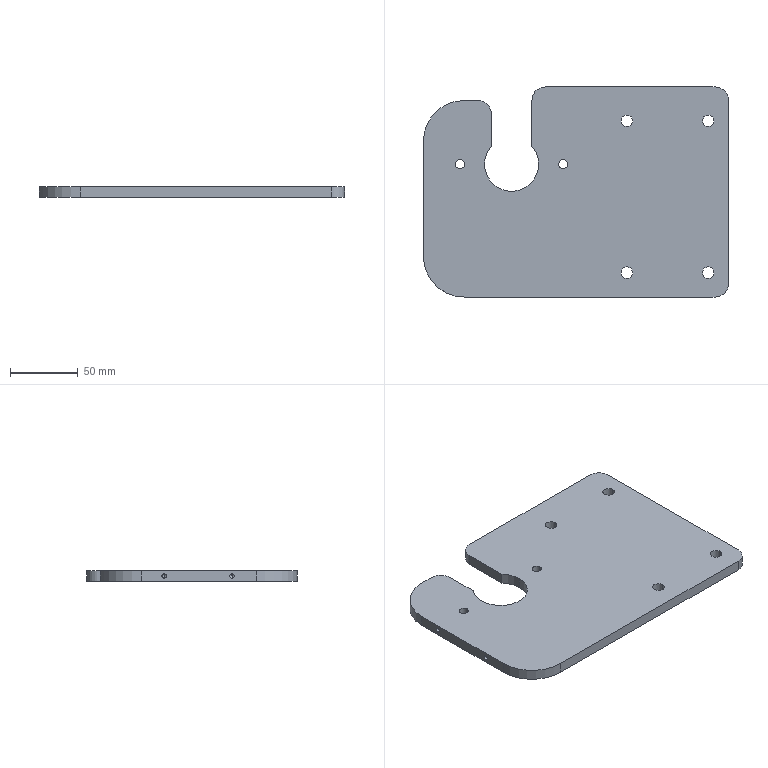Part | SolidWorks | features BaseBody 1 | 1 solid | 38 faces | box 225 x 155 x 8 mm | volume 249192 mm3 | cylinder 25 | plane 9 | cone 4 | commonest cylinder face diameters 8.5 x8 3.3 x4 6.8 x4 20 x4 40 x3 60 x2
STEP:
#1=CARTESIAN_POINT('',(-67.5,20.5,0.));
#2=VERTEX_POINT('',#1);
#3=CARTESIAN_POINT('',(-27.5,20.5,0.));
#4=VERTEX_POINT('',#3);
#5=CARTESIAN_POINT('',(-47.5,20.5,0.));
#6=DIRECTION('',(0.,0.,1.));
#7=DIRECTION('',(1.,0.,0.));
#8=AXIS2_PLACEMENT_3D('',#5,#6,#7);
#9=CIRCLE('',#8,20.);
#10=EDGE_CURVE('',#2,#4,#9,.T.);
#11=ORIENTED_EDGE('',*,*,#10,.F.);
#12=CARTESIAN_POINT('',(-67.5,20.5,8.));
#13=VERTEX_POINT('',#12);
#14=CARTESIAN_POINT('',(-67.5,20.5,0.));
#15=DIRECTION('',(0.,0.,1.));
#16=VECTOR('',#15,1000.);
#17=LINE('',#14,#16);
#18=EDGE_CURVE('',#2,#13,#17,.T.);
#19=ORIENTED_EDGE('',*,*,#18,.T.);
#20=CARTESIAN_POINT('',(-27.5,20.5,8.));
#21=VERTEX_POINT('',#20);
#22=CARTESIAN_POINT('',(-47.5,20.5,8.));
#23=DIRECTION('',(0.,0.,1.));
#24=DIRECTION('',(1.,0.,0.));
#25=AXIS2_PLACEMENT_3D('',#22,#23,#24);
#26=CIRCLE('',#25,20.);
#27=EDGE_CURVE('',#13,#21,#26,.T.);
#28=ORIENTED_EDGE('',*,*,#27,.T.);
#29=CARTESIAN_POINT('',(-27.5,20.5,0.));
#30=DIRECTION('',(0.,0.,1.));
#31=VECTOR('',#30,1000.);
#32=LINE('',#29,#31);
#33=EDGE_CURVE('',#4,#21,#32,.T.);
#34=ORIENTED_EDGE('',*,*,#33,.F.);
#35=EDGE_LOOP('',(#11,#19,#28,#34));
#36=FACE_OUTER_BOUND('',#35,.T.);
#37=CARTESIAN_POINT('',(-47.5,20.5,0.));
#38=DIRECTION('',(0.,0.,1.));
#39=DIRECTION('',(1.,0.,0.));
#40=AXIS2_PLACEMENT_3D('',#37,#38,#39);
#41=CYLINDRICAL_SURFACE('',#40,20.);
#42=ADVANCED_FACE('',(#36),#41,.F.);
#43=CARTESIAN_POINT('',(-32.5,33.729,0.));
#44=VERTEX_POINT('',#43);
#45=CARTESIAN_POINT('',(-47.5,20.5,0.));
#46=DIRECTION('',(0.,0.,1.));
#47=DIRECTION('',(1.,0.,0.));
#48=AXIS2_PLACEMENT_3D('',#45,#46,#47);
#49=CIRCLE('',#48,20.);
#50=EDGE_CURVE('',#4,#44,#49,.T.);
#51=ORIENTED_EDGE('',*,*,#50,.F.);
#52=ORIENTED_EDGE('',*,*,#33,.T.);
#53=CARTESIAN_POINT('',(-32.5,33.729,8.));
#54=VERTEX_POINT('',#53);
#55=CARTESIAN_POINT('',(-47.5,20.5,8.));
#56=DIRECTION('',(0.,0.,1.));
#57=DIRECTION('',(1.,0.,0.));
#58=AXIS2_PLACEMENT_3D('',#55,#56,#57);
#59=CIRCLE('',#58,20.);
#60=EDGE_CURVE('',#21,#54,#59,.T.);
#61=ORIENTED_EDGE('',*,*,#60,.T.);
#62=CARTESIAN_POINT('',(-32.5,33.729,8.));
#63=DIRECTION('',(0.,0.,-1.));
#64=VECTOR('',#63,1000.);
#65=LINE('',#62,#64);
#66=EDGE_CURVE('',#54,#44,#65,.T.);
#67=ORIENTED_EDGE('',*,*,#66,.T.);
#68=EDGE_LOOP('',(#51,#52,#61,#67));
#69=FACE_OUTER_BOUND('',#68,.T.);
#70=CARTESIAN_POINT('',(-47.5,20.5,0.));
#71=DIRECTION('',(0.,0.,1.));
#72=DIRECTION('',(1.,0.,0.));
#73=AXIS2_PLACEMENT_3D('',#70,#71,#72);
#74=CYLINDRICAL_SURFACE('',#73,20.);
#75=ADVANCED_FACE('',(#69),#74,.F.);
#76=CARTESIAN_POINT('',(33.25,52.5,8.));
#77=VERTEX_POINT('',#76);
#78=CARTESIAN_POINT('',(41.75,52.5,8.));
#79=VERTEX_POINT('',#78);
#80=CARTESIAN_POINT('',(37.5,52.5,8.));
#81=DIRECTION('',(0.,0.,1.));
#82=DIRECTION('',(-1.,0.,0.));
#83=AXIS2_PLACEMENT_3D('',#80,#81,#82);
#84=CIRCLE('',#83,4.25);
#85=EDGE_CURVE('',#77,#79,#84,.T.);
#86=ORIENTED_EDGE('',*,*,#85,.T.);
#87=CARTESIAN_POINT('',(41.75,52.5,0.));
#88=VERTEX_POINT('',#87);
#89=CARTESIAN_POINT('',(41.75,52.5,0.));
#90=DIRECTION('',(0.,0.,-1.));
#91=VECTOR('',#90,1000.);
#92=LINE('',#89,#91);
#93=EDGE_CURVE('',#79,#88,#92,.T.);
#94=ORIENTED_EDGE('',*,*,#93,.T.);
#95=CARTESIAN_POINT('',(33.25,52.5,0.));
#96=VERTEX_POINT('',#95);
#97=CARTESIAN_POINT('',(37.5,52.5,0.));
#98=DIRECTION('',(0.,0.,1.));
#99=DIRECTION('',(-1.,0.,0.));
#100=AXIS2_PLACEMENT_3D('',#97,#98,#99);
#101=CIRCLE('',#100,4.25);
#102=EDGE_CURVE('',#96,#88,#101,.T.);
#103=ORIENTED_EDGE('',*,*,#102,.F.);
#104=CARTESIAN_POINT('',(33.25,52.5,0.));
#105=DIRECTION('',(0.,0.,-1.));
#106=VECTOR('',#105,1000.);
#107=LINE('',#104,#106);
#108=EDGE_CURVE('',#77,#96,#107,.T.);
#109=ORIENTED_EDGE('',*,*,#108,.F.);
#110=EDGE_LOOP('',(#86,#94,#103,#109));
#111=FACE_OUTER_BOUND('',#110,.T.);
#112=CARTESIAN_POINT('',(37.5,52.5,0.));
#113=DIRECTION('',(0.,0.,-1.));
#114=DIRECTION('',(-1.,0.,0.));
#115=AXIS2_PLACEMENT_3D('',#112,#113,#114);
#116=CYLINDRICAL_SURFACE('',#115,4.25);
#117=ADVANCED_FACE('',(#111),#116,.F.);
#118=CARTESIAN_POINT('',(93.25,-59.5,8.));
#119=VERTEX_POINT('',#118);
#120=CARTESIAN_POINT('',(101.75,-59.5,8.));
#121=VERTEX_POINT('',#120);
#122=CARTESIAN_POINT('',(97.5,-59.5,8.));
#123=DIRECTION('',(0.,0.,1.));
#124=DIRECTION('',(-1.,0.,0.));
#125=AXIS2_PLACEMENT_3D('',#122,#123,#124);
#126=CIRCLE('',#125,4.25);
#127=EDGE_CURVE('',#119,#121,#126,.T.);
#128=ORIENTED_EDGE('',*,*,#127,.T.);
#129=CARTESIAN_POINT('',(101.75,-59.5,0.));
#130=VERTEX_POINT('',#129);
#131=CARTESIAN_POINT('',(101.75,-59.5,0.));
#132=DIRECTION('',(0.,0.,-1.));
#133=VECTOR('',#132,1000.);
#134=LINE('',#131,#133);
#135=EDGE_CURVE('',#121,#130,#134,.T.);
#136=ORIENTED_EDGE('',*,*,#135,.T.);
#137=CARTESIAN_POINT('',(93.25,-59.5,0.));
#138=VERTEX_POINT('',#137);
#139=CARTESIAN_POINT('',(97.5,-59.5,0.));
#140=DIRECTION('',(0.,0.,1.));
#141=DIRECTION('',(-1.,0.,0.));
#142=AXIS2_PLACEMENT_3D('',#139,#140,#141);
#143=CIRCLE('',#142,4.25);
#144=EDGE_CURVE('',#138,#130,#143,.T.);
#145=ORIENTED_EDGE('',*,*,#144,.F.);
#146=CARTESIAN_POINT('',(93.25,-59.5,0.));
#147=DIRECTION('',(0.,0.,-1.));
#148=VECTOR('',#147,1000.);
#149=LINE('',#146,#148);
#150=EDGE_CURVE('',#119,#138,#149,.T.);
#151=ORIENTED_EDGE('',*,*,#150,.F.);
#152=EDGE_LOOP('',(#128,#136,#145,#151));
#153=FACE_OUTER_BOUND('',#152,.T.);
#154=CARTESIAN_POINT('',(97.5,-59.5,0.));
#155=DIRECTION('',(0.,0.,-1.));
#156=DIRECTION('',(-1.,0.,0.));
#157=AXIS2_PLACEMENT_3D('',#154,#155,#156);
#158=CYLINDRICAL_SURFACE('',#157,4.25);
#159=ADVANCED_FACE('',(#153),#158,.F.);
#160=CARTESIAN_POINT('',(33.25,-59.5,8.));
#161=VERTEX_POINT('',#160);
#162=CARTESIAN_POINT('',(41.75,-59.5,8.));
#163=VERTEX_POINT('',#162);
#164=CARTESIAN_POINT('',(37.5,-59.5,8.));
#165=DIRECTION('',(0.,0.,1.));
#166=DIRECTION('',(-1.,0.,0.));
#167=AXIS2_PLACEMENT_3D('',#164,#165,#166);
#168=CIRCLE('',#167,4.25);
#169=EDGE_CURVE('',#161,#163,#168,.T.);
#170=ORIENTED_EDGE('',*,*,#169,.T.);
#171=CARTESIAN_POINT('',(41.75,-59.5,0.));
#172=VERTEX_POINT('',#171);
#173=CARTESIAN_POINT('',(41.75,-59.5,0.));
#174=DIRECTION('',(0.,0.,-1.));
#175=VECTOR('',#174,1000.);
#176=LINE('',#173,#175);
#177=EDGE_CURVE('',#163,#172,#176,.T.);
#178=ORIENTED_EDGE('',*,*,#177,.T.);
#179=CARTESIAN_POINT('',(33.25,-59.5,0.));
#180=VERTEX_POINT('',#179);
#181=CARTESIAN_POINT('',(37.5,-59.5,0.));
#182=DIRECTION('',(0.,0.,1.));
#183=DIRECTION('',(-1.,0.,0.));
#184=AXIS2_PLACEMENT_3D('',#181,#182,#183);
#185=CIRCLE('',#184,4.25);
#186=EDGE_CURVE('',#180,#172,#185,.T.);
#187=ORIENTED_EDGE('',*,*,#186,.F.);
#188=CARTESIAN_POINT('',(33.25,-59.5,0.));
#189=DIRECTION('',(0.,0.,-1.));
#190=VECTOR('',#189,1000.);
#191=LINE('',#188,#190);
#192=EDGE_CURVE('',#161,#180,#191,.T.);
#193=ORIENTED_EDGE('',*,*,#192,.F.);
#194=EDGE_LOOP('',(#170,#178,#187,#193));
#195=FACE_OUTER_BOUND('',#194,.T.);
#196=CARTESIAN_POINT('',(37.5,-59.5,0.));
#197=DIRECTION('',(0.,0.,-1.));
#198=DIRECTION('',(-1.,0.,0.));
#199=AXIS2_PLACEMENT_3D('',#196,#197,#198);
#200=CYLINDRICAL_SURFACE('',#199,4.25);
#201=ADVANCED_FACE('',(#195),#200,.F.);
#202=CARTESIAN_POINT('',(93.25,52.5,8.));
#203=VERTEX_POINT('',#202);
#204=CARTESIAN_POINT('',(101.75,52.5,8.));
#205=VERTEX_POINT('',#204);
#206=CARTESIAN_POINT('',(97.5,52.5,8.));
#207=DIRECTION('',(0.,0.,1.));
#208=DIRECTION('',(-1.,0.,0.));
#209=AXIS2_PLACEMENT_3D('',#206,#207,#208);
#210=CIRCLE('',#209,4.25);
#211=EDGE_CURVE('',#203,#205,#210,.T.);
#212=ORIENTED_EDGE('',*,*,#211,.T.);
#213=CARTESIAN_POINT('',(101.75,52.5,0.));
#214=VERTEX_POINT('',#213);
#215=CARTESIAN_POINT('',(101.75,52.5,0.));
#216=DIRECTION('',(0.,0.,-1.));
#217=VECTOR('',#216,1000.);
#218=LINE('',#215,#217);
#219=EDGE_CURVE('',#205,#214,#218,.T.);
#220=ORIENTED_EDGE('',*,*,#219,.T.);
#221=CARTESIAN_POINT('',(93.25,52.5,0.));
#222=VERTEX_POINT('',#221);
#223=CARTESIAN_POINT('',(97.5,52.5,0.));
#224=DIRECTION('',(0.,0.,1.));
#225=DIRECTION('',(-1.,0.,0.));
#226=AXIS2_PLACEMENT_3D('',#223,#224,#225);
#227=CIRCLE('',#226,4.25);
#228=EDGE_CURVE('',#222,#214,#227,.T.);
#229=ORIENTED_EDGE('',*,*,#228,.F.);
#230=CARTESIAN_POINT('',(93.25,52.5,0.));
#231=DIRECTION('',(0.,0.,-1.));
#232=VECTOR('',#231,1000.);
#233=LINE('',#230,#232);
#234=EDGE_CURVE('',#203,#222,#233,.T.);
#235=ORIENTED_EDGE('',*,*,#234,.F.);
#236=EDGE_LOOP('',(#212,#220,#229,#235));
#237=FACE_OUTER_BOUND('',#236,.T.);
#238=CARTESIAN_POINT('',(97.5,52.5,0.));
#239=DIRECTION('',(0.,0.,-1.));
#240=DIRECTION('',(-1.,0.,0.));
#241=AXIS2_PLACEMENT_3D('',#238,#239,#240);
#242=CYLINDRICAL_SURFACE('',#241,4.25);
#243=ADVANCED_FACE('',(#237),#242,.F.);
#244=CARTESIAN_POINT('',(-88.9,20.5,8.));
#245=VERTEX_POINT('',#244);
#246=CARTESIAN_POINT('',(-82.1,20.5,8.));
#247=VERTEX_POINT('',#246);
#248=CARTESIAN_POINT('',(-85.5,20.5,8.));
#249=DIRECTION('',(0.,0.,1.));
#250=DIRECTION('',(-1.,0.,0.));
#251=AXIS2_PLACEMENT_3D('',#248,#249,#250);
#252=CIRCLE('',#251,3.4);
#253=EDGE_CURVE('',#245,#247,#252,.T.);
#254=ORIENTED_EDGE('',*,*,#253,.T.);
#255=CARTESIAN_POINT('',(-82.1,20.5,0.));
#256=VERTEX_POINT('',#255);
#257=CARTESIAN_POINT('',(-82.1,20.5,0.));
#258=DIRECTION('',(0.,0.,-1.));
#259=VECTOR('',#258,1000.);
#260=LINE('',#257,#259);
#261=EDGE_CURVE('',#247,#256,#260,.T.);
#262=ORIENTED_EDGE('',*,*,#261,.T.);
#263=CARTESIAN_POINT('',(-88.9,20.5,0.));
#264=VERTEX_POINT('',#263);
#265=CARTESIAN_POINT('',(-85.5,20.5,0.));
#266=DIRECTION('',(0.,0.,1.));
#267=DIRECTION('',(-1.,0.,0.));
#268=AXIS2_PLACEMENT_3D('',#265,#266,#267);
#269=CIRCLE('',#268,3.4);
#270=EDGE_CURVE('',#264,#256,#269,.T.);
#271=ORIENTED_EDGE('',*,*,#270,.F.);
#272=CARTESIAN_POINT('',(-88.9,20.5,0.));
#273=DIRECTION('',(0.,0.,-1.));
#274=VECTOR('',#273,1000.);
#275=LINE('',#272,#274);
#276=EDGE_CURVE('',#245,#264,#275,.T.);
#277=ORIENTED_EDGE('',*,*,#276,.F.);
#278=EDGE_LOOP('',(#254,#262,#271,#277));
#279=FACE_OUTER_BOUND('',#278,.T.);
#280=CARTESIAN_POINT('',(-85.5,20.5,0.));
#281=DIRECTION('',(0.,0.,-1.));
#282=DIRECTION('',(-1.,0.,0.));
#283=AXIS2_PLACEMENT_3D('',#280,#281,#282);
#284=CYLINDRICAL_SURFACE('',#283,3.4);
#285=ADVANCED_FACE('',(#279),#284,.F.);
#286=CARTESIAN_POINT('',(-12.9,20.5,8.));
#287=VERTEX_POINT('',#286);
#288=CARTESIAN_POINT('',(-6.1,20.5,8.));
#289=VERTEX_POINT('',#288);
#290=CARTESIAN_POINT('',(-9.5,20.5,8.));
#291=DIRECTION('',(0.,0.,1.));
#292=DIRECTION('',(-1.,0.,0.));
#293=AXIS2_PLACEMENT_3D('',#290,#291,#292);
#294=CIRCLE('',#293,3.4);
#295=EDGE_CURVE('',#287,#289,#294,.T.);
#296=ORIENTED_EDGE('',*,*,#295,.T.);
#297=CARTESIAN_POINT('',(-6.1,20.5,0.));
#298=VERTEX_POINT('',#297);
#299=CARTESIAN_POINT('',(-6.1,20.5,0.));
#300=DIRECTION('',(0.,0.,-1.));
#301=VECTOR('',#300,1000.);
#302=LINE('',#299,#301);
#303=EDGE_CURVE('',#289,#298,#302,.T.);
#304=ORIENTED_EDGE('',*,*,#303,.T.);
#305=CARTESIAN_POINT('',(-12.9,20.5,0.));
#306=VERTEX_POINT('',#305);
#307=CARTESIAN_POINT('',(-9.5,20.5,0.));
#308=DIRECTION('',(0.,0.,1.));
#309=DIRECTION('',(-1.,0.,0.));
#310=AXIS2_PLACEMENT_3D('',#307,#308,#309);
#311=CIRCLE('',#310,3.4);
#312=EDGE_CURVE('',#306,#298,#311,.T.);
#313=ORIENTED_EDGE('',*,*,#312,.F.);
#314=CARTESIAN_POINT('',(-12.9,20.5,0.));
#315=DIRECTION('',(0.,0.,-1.));
#316=VECTOR('',#315,1000.);
#317=LINE('',#314,#316);
#318=EDGE_CURVE('',#287,#306,#317,.T.);
#319=ORIENTED_EDGE('',*,*,#318,.F.);
#320=EDGE_LOOP('',(#296,#304,#313,#319));
#321=FACE_OUTER_BOUND('',#320,.T.);
#322=CARTESIAN_POINT('',(-9.5,20.5,0.));
#323=DIRECTION('',(0.,0.,-1.));
#324=DIRECTION('',(-1.,0.,0.));
#325=AXIS2_PLACEMENT_3D('',#322,#323,#324);
#326=CYLINDRICAL_SURFACE('',#325,3.4);
#327=ADVANCED_FACE('',(#321),#326,.F.);
#328=CARTESIAN_POINT('',(-101.,-29.5,2.35));
#329=VERTEX_POINT('',#328);
#330=CARTESIAN_POINT('',(-101.,-29.5,5.65));
#331=VERTEX_POINT('',#330);
#332=CARTESIAN_POINT('',(-101.,-29.5,4.));
#333=DIRECTION('',(-1.,0.,0.));
#334=DIRECTION('',(0.,0.,1.));
#335=AXIS2_PLACEMENT_3D('',#332,#333,#334);
#336=CIRCLE('',#335,1.65);
#337=EDGE_CURVE('',#329,#331,#336,.T.);
#338=ORIENTED_EDGE('',*,*,#337,.F.);
#339=CARTESIAN_POINT('',(-112.5,-29.5,2.35));
#340=VERTEX_POINT('',#339);
#341=CARTESIAN_POINT('',(-112.5,-29.5,2.35));
#342=DIRECTION('',(-1.,0.,0.));
#343=VECTOR('',#342,1000.);
#344=LINE('',#341,#343);
#345=EDGE_CURVE('',#329,#340,#344,.T.);
#346=ORIENTED_EDGE('',*,*,#345,.T.);
#347=CARTESIAN_POINT('',(-112.5,-29.5,5.65));
#348=VERTEX_POINT('',#347);
#349=CARTESIAN_POINT('',(-112.5,-29.5,4.));
#350=DIRECTION('',(-1.,0.,0.));
#351=DIRECTION('',(0.,0.,1.));
#352=AXIS2_PLACEMENT_3D('',#349,#350,#351);
#353=CIRCLE('',#352,1.65);
#354=EDGE_CURVE('',#340,#348,#353,.T.);
#355=ORIENTED_EDGE('',*,*,#354,.T.);
#356=CARTESIAN_POINT('',(-112.5,-29.5,5.65));
#357=DIRECTION('',(-1.,0.,0.));
#358=VECTOR('',#357,1000.);
#359=LINE('',#356,#358);
#360=EDGE_CURVE('',#331,#348,#359,.T.);
#361=ORIENTED_EDGE('',*,*,#360,.F.);
#362=EDGE_LOOP('',(#338,#346,#355,#361));
#363=FACE_OUTER_BOUND('',#362,.T.);
#364=CARTESIAN_POINT('',(-112.5,-29.5,4.));
#365=DIRECTION('',(-1.,0.,0.));
#366=DIRECTION('',(0.,0.,1.));
#367=AXIS2_PLACEMENT_3D('',#364,#365,#366);
#368=CYLINDRICAL_SURFACE('',#367,1.65);
#369=ADVANCED_FACE('',(#363),#368,.F.);
#370=CARTESIAN_POINT('',(-101.,20.5,2.35));
#371=VERTEX_POINT('',#370);
#372=CARTESIAN_POINT('',(-101.,20.5,5.65));
#373=VERTEX_POINT('',#372);
#374=CARTESIAN_POINT('',(-101.,20.5,4.));
#375=DIRECTION('',(-1.,0.,0.));
#376=DIRECTION('',(0.,0.,1.));
#377=AXIS2_PLACEMENT_3D('',#374,#375,#376);
#378=CIRCLE('',#377,1.65);
#379=EDGE_CURVE('',#371,#373,#378,.T.);
#380=ORIENTED_EDGE('',*,*,#379,.F.);
#381=CARTESIAN_POINT('',(-112.5,20.5,2.35));
#382=VERTEX_POINT('',#381);
#383=CARTESIAN_POINT('',(-112.5,20.5,2.35));
#384=DIRECTION('',(-1.,0.,0.));
#385=VECTOR('',#384,1000.);
#386=LINE('',#383,#385);
#387=EDGE_CURVE('',#371,#382,#386,.T.);
#388=ORIENTED_EDGE('',*,*,#387,.T.);
#389=CARTESIAN_POINT('',(-112.5,20.5,5.65));
#390=VERTEX_POINT('',#389);
#391=CARTESIAN_POINT('',(-112.5,20.5,4.));
#392=DIRECTION('',(-1.,0.,0.));
#393=DIRECTION('',(0.,0.,1.));
#394=AXIS2_PLACEMENT_3D('',#391,#392,#393);
#395=CIRCLE('',#394,1.65);
#396=EDGE_CURVE('',#382,#390,#395,.T.);
#397=ORIENTED_EDGE('',*,*,#396,.T.);
#398=CARTESIAN_POINT('',(-112.5,20.5,5.65));
#399=DIRECTION('',(-1.,0.,0.));
#400=VECTOR('',#399,1000.);
#401=LINE('',#398,#400);
#402=EDGE_CURVE('',#373,#390,#401,.T.);
#403=ORIENTED_EDGE('',*,*,#402,.F.);
#404=EDGE_LOOP('',(#380,#388,#397,#403));
#405=FACE_OUTER_BOUND('',#404,.T.);
#406=CARTESIAN_POINT('',(-112.5,20.5,4.));
#407=DIRECTION('',(-1.,0.,0.));
#408=DIRECTION('',(0.,0.,1.));
#409=AXIS2_PLACEMENT_3D('',#406,#407,#408);
#410=CYLINDRICAL_SURFACE('',#409,1.65);
#411=ADVANCED_FACE('',(#405),#410,.F.);
#412=CARTESIAN_POINT('',(-100.009,-29.5,4.));
#413=VERTEX_POINT('',#412);
#414=CARTESIAN_POINT('',(-101.,-29.5,5.65));
#415=DIRECTION('',(-0.515,0.,0.8572));
#416=VECTOR('',#415,1000.);
#417=LINE('',#414,#416);
#418=EDGE_CURVE('',#413,#331,#417,.T.);
#419=ORIENTED_EDGE('',*,*,#418,.F.);
#420=CARTESIAN_POINT('',(-101.,-29.5,2.35));
#421=DIRECTION('',(-0.515,0.,-0.8572));
#422=VECTOR('',#421,1000.);
#423=LINE('',#420,#422);
#424=EDGE_CURVE('',#413,#329,#423,.T.);
#425=ORIENTED_EDGE('',*,*,#424,.T.);
#426=ORIENTED_EDGE('',*,*,#337,.T.);
#427=EDGE_LOOP('',(#419,#425,#426));
#428=FACE_OUTER_BOUND('',#427,.T.);
#429=CARTESIAN_POINT('',(-101.,-29.5,4.));
#430=DIRECTION('',(-1.,0.,0.));
#431=DIRECTION('',(0.,0.,1.));
#432=AXIS2_PLACEMENT_3D('',#429,#430,#431);
#433=CONICAL_SURFACE('',#432,1.65,1.03);
#434=ADVANCED_FACE('',(#428),#433,.F.);
#435=CARTESIAN_POINT('',(-100.009,20.5,4.));
#436=VERTEX_POINT('',#435);
#437=CARTESIAN_POINT('',(-101.,20.5,5.65));
#438=DIRECTION('',(-0.515,0.,0.8572));
#439=VECTOR('',#438,1000.);
#440=LINE('',#437,#439);
#441=EDGE_CURVE('',#436,#373,#440,.T.);
#442=ORIENTED_EDGE('',*,*,#441,.F.);
#443=CARTESIAN_POINT('',(-101.,20.5,2.35));
#444=DIRECTION('',(-0.515,0.,-0.8572));
#445=VECTOR('',#444,1000.);
#446=LINE('',#443,#445);
#447=EDGE_CURVE('',#436,#371,#446,.T.);
#448=ORIENTED_EDGE('',*,*,#447,.T.);
#449=ORIENTED_EDGE('',*,*,#379,.T.);
#450=EDGE_LOOP('',(#442,#448,#449));
#451=FACE_OUTER_BOUND('',#450,.T.);
#452=CARTESIAN_POINT('',(-101.,20.5,4.));
#453=DIRECTION('',(-1.,0.,0.));
#454=DIRECTION('',(0.,0.,1.));
#455=AXIS2_PLACEMENT_3D('',#452,#453,#454);
#456=CONICAL_SURFACE('',#455,1.65,1.03);
#457=ADVANCED_FACE('',(#451),#456,.F.);
#458=CARTESIAN_POINT('',(112.5,-67.5,8.));
#459=VERTEX_POINT('',#458);
#460=CARTESIAN_POINT('',(102.5,-77.5,8.));
#461=VERTEX_POINT('',#460);
#462=CARTESIAN_POINT('',(102.5,-67.5,8.));
#463=DIRECTION('',(0.,0.,-1.));
#464=DIRECTION('',(-1.,0.,0.));
#465=AXIS2_PLACEMENT_3D('',#462,#463,#464);
#466=CIRCLE('',#465,10.);
#467=EDGE_CURVE('',#459,#461,#466,.T.);
#468=ORIENTED_EDGE('',*,*,#467,.F.);
#469=CARTESIAN_POINT('',(112.5,67.5,8.));
#470=VERTEX_POINT('',#469);
#471=CARTESIAN_POINT('',(112.5,0.,8.));
#472=DIRECTION('',(0.,-1.,0.));
#473=VECTOR('',#472,1000.);
#474=LINE('',#471,#473);
#475=EDGE_CURVE('',#470,#459,#474,.T.);
#476=ORIENTED_EDGE('',*,*,#475,.F.);
#477=CARTESIAN_POINT('',(102.5,77.5,8.));
#478=VERTEX_POINT('',#477);
#479=CARTESIAN_POINT('',(102.5,67.5,8.));
#480=DIRECTION('',(0.,0.,-1.));
#481=DIRECTION('',(-1.,0.,0.));
#482=AXIS2_PLACEMENT_3D('',#479,#480,#481);
#483=CIRCLE('',#482,10.);
#484=EDGE_CURVE('',#478,#470,#483,.T.);
#485=ORIENTED_EDGE('',*,*,#484,.F.);
#486=CARTESIAN_POINT('',(-22.5,77.5,8.));
#487=VERTEX_POINT('',#486);
#488=CARTESIAN_POINT('',(0.,77.5,8.));
#489=DIRECTION('',(1.,0.,0.));
#490=VECTOR('',#489,1000.);
#491=LINE('',#488,#490);
#492=EDGE_CURVE('',#487,#478,#491,.T.);
#493=ORIENTED_EDGE('',*,*,#492,.F.);
#494=CARTESIAN_POINT('',(-32.5,67.5,8.));
#495=VERTEX_POINT('',#494);
#496=CARTESIAN_POINT('',(-22.5,67.5,8.));
#497=DIRECTION('',(0.,0.,-1.));
#498=DIRECTION('',(1.,0.,0.));
#499=AXIS2_PLACEMENT_3D('',#496,#497,#498);
#500=CIRCLE('',#499,10.);
#501=EDGE_CURVE('',#495,#487,#500,.T.);
#502=ORIENTED_EDGE('',*,*,#501,.F.);
#503=CARTESIAN_POINT('',(-32.5,0.,8.));
#504=DIRECTION('',(0.,1.,0.));
#505=VECTOR('',#504,1000.);
#506=LINE('',#503,#505);
#507=EDGE_CURVE('',#54,#495,#506,.T.);
#508=ORIENTED_EDGE('',*,*,#507,.F.);
#509=ORIENTED_EDGE('',*,*,#60,.F.);
#510=ORIENTED_EDGE('',*,*,#27,.F.);
#511=CARTESIAN_POINT('',(-62.5,33.729,8.));
#512=VERTEX_POINT('',#511);
#513=CARTESIAN_POINT('',(-47.5,20.5,8.));
#514=DIRECTION('',(0.,0.,1.));
#515=DIRECTION('',(1.,0.,0.));
#516=AXIS2_PLACEMENT_3D('',#513,#514,#515);
#517=CIRCLE('',#516,20.);
#518=EDGE_CURVE('',#512,#13,#517,.T.);
#519=ORIENTED_EDGE('',*,*,#518,.F.);
#520=CARTESIAN_POINT('',(-62.5,57.5,8.));
#521=VERTEX_POINT('',#520);
#522=CARTESIAN_POINT('',(-62.5,0.,8.));
#523=DIRECTION('',(0.,-1.,0.));
#524=VECTOR('',#523,1000.);
#525=LINE('',#522,#524);
#526=EDGE_CURVE('',#521,#512,#525,.T.);
#527=ORIENTED_EDGE('',*,*,#526,.F.);
#528=CARTESIAN_POINT('',(-72.5,67.5,8.));
#529=VERTEX_POINT('',#528);
#530=CARTESIAN_POINT('',(-72.5,57.5,8.));
#531=DIRECTION('',(0.,0.,-1.));
#532=DIRECTION('',(1.,0.,0.));
#533=AXIS2_PLACEMENT_3D('',#530,#531,#532);
#534=CIRCLE('',#533,10.);
#535=EDGE_CURVE('',#529,#521,#534,.T.);
#536=ORIENTED_EDGE('',*,*,#535,.F.);
#537=CARTESIAN_POINT('',(-82.5,67.5,8.));
#538=VERTEX_POINT('',#537);
#539=CARTESIAN_POINT('',(0.,67.5,8.));
#540=DIRECTION('',(1.,0.,0.));
#541=VECTOR('',#540,1000.);
#542=LINE('',#539,#541);
#543=EDGE_CURVE('',#538,#529,#542,.T.);
#544=ORIENTED_EDGE('',*,*,#543,.F.);
#545=CARTESIAN_POINT('',(-112.5,37.5,8.));
#546=VERTEX_POINT('',#545);
#547=CARTESIAN_POINT('',(-82.5,37.5,8.));
#548=DIRECTION('',(0.,0.,-1.));
#549=DIRECTION('',(1.,0.,0.));
#550=AXIS2_PLACEMENT_3D('',#547,#548,#549);
#551=CIRCLE('',#550,30.);
#552=EDGE_CURVE('',#546,#538,#551,.T.);
#553=ORIENTED_EDGE('',*,*,#552,.F.);
#554=CARTESIAN_POINT('',(-112.5,-47.5,8.));
#555=VERTEX_POINT('',#554);
#556=CARTESIAN_POINT('',(-112.5,0.,8.));
#557=DIRECTION('',(0.,1.,0.));
#558=VECTOR('',#557,1000.);
#559=LINE('',#556,#558);
#560=EDGE_CURVE('',#555,#546,#559,.T.);
#561=ORIENTED_EDGE('',*,*,#560,.F.);
#562=CARTESIAN_POINT('',(-82.5,-77.5,8.));
#563=VERTEX_POINT('',#562);
#564=CARTESIAN_POINT('',(-82.5,-47.5,8.));
#565=DIRECTION('',(0.,0.,-1.));
#566=DIRECTION('',(-1.,0.,0.));
#567=AXIS2_PLACEMENT_3D('',#564,#565,#566);
#568=CIRCLE('',#567,30.);
#569=EDGE_CURVE('',#563,#555,#568,.T.);
#570=ORIENTED_EDGE('',*,*,#569,.F.);
#571=CARTESIAN_POINT('',(0.,-77.5,8.));
#572=DIRECTION('',(-1.,0.,0.));
#573=VECTOR('',#572,1000.);
#574=LINE('',#571,#573);
#575=EDGE_CURVE('',#461,#563,#574,.T.);
#576=ORIENTED_EDGE('',*,*,#575,.F.);
#577=EDGE_LOOP('',(#468,#476,#485,#493,#502,#508,#509,#510,#519,#527,#536,#544,#553,#561,#570,#576));
#578=FACE_OUTER_BOUND('',#577,.T.);
#579=ORIENTED_EDGE('',*,*,#85,.F.);
#580=CARTESIAN_POINT('',(37.5,52.5,8.));
#581=DIRECTION('',(0.,0.,1.));
#582=DIRECTION('',(-1.,0.,0.));
#583=AXIS2_PLACEMENT_3D('',#580,#581,#582);
#584=CIRCLE('',#583,4.25);
#585=EDGE_CURVE('',#79,#77,#584,.T.);
#586=ORIENTED_EDGE('',*,*,#585,.F.);
#587=EDGE_LOOP('',(#579,#586));
#588=FACE_BOUND('',#587,.T.);
#589=ORIENTED_EDGE('',*,*,#127,.F.);
#590=CARTESIAN_POINT('',(97.5,-59.5,8.));
#591=DIRECTION('',(0.,0.,1.));
#592=DIRECTION('',(-1.,0.,0.));
#593=AXIS2_PLACEMENT_3D('',#590,#591,#592);
#594=CIRCLE('',#593,4.25);
#595=EDGE_CURVE('',#121,#119,#594,.T.);
#596=ORIENTED_EDGE('',*,*,#595,.F.);
#597=EDGE_LOOP('',(#589,#596));
#598=FACE_BOUND('',#597,.T.);
#599=ORIENTED_EDGE('',*,*,#169,.F.);
#600=CARTESIAN_POINT('',(37.5,-59.5,8.));
#601=DIRECTION('',(0.,0.,1.));
#602=DIRECTION('',(-1.,0.,0.));
#603=AXIS2_PLACEMENT_3D('',#600,#601,#602);
#604=CIRCLE('',#603,4.25);
#605=EDGE_CURVE('',#163,#161,#604,.T.);
#606=ORIENTED_EDGE('',*,*,#605,.F.);
#607=EDGE_LOOP('',(#599,#606));
#608=FACE_BOUND('',#607,.T.);
#609=ORIENTED_EDGE('',*,*,#211,.F.);
#610=CARTESIAN_POINT('',(97.5,52.5,8.));
#611=DIRECTION('',(0.,0.,1.));
#612=DIRECTION('',(-1.,0.,0.));
#613=AXIS2_PLACEMENT_3D('',#610,#611,#612);
#614=CIRCLE('',#613,4.25);
#615=EDGE_CURVE('',#205,#203,#614,.T.);
#616=ORIENTED_EDGE('',*,*,#615,.F.);
#617=EDGE_LOOP('',(#609,#616));
#618=FACE_BOUND('',#617,.T.);
#619=ORIENTED_EDGE('',*,*,#253,.F.);
#620=CARTESIAN_POINT('',(-85.5,20.5,8.));
#621=DIRECTION('',(0.,0.,1.));
#622=DIRECTION('',(-1.,0.,0.));
#623=AXIS2_PLACEMENT_3D('',#620,#621,#622);
#624=CIRCLE('',#623,3.4);
#625=EDGE_CURVE('',#247,#245,#624,.T.);
#626=ORIENTED_EDGE('',*,*,#625,.F.);
#627=EDGE_LOOP('',(#619,#626));
#628=FACE_BOUND('',#627,.T.);
#629=ORIENTED_EDGE('',*,*,#295,.F.);
#630=CARTESIAN_POINT('',(-9.5,20.5,8.));
#631=DIRECTION('',(0.,0.,1.));
#632=DIRECTION('',(-1.,0.,0.));
#633=AXIS2_PLACEMENT_3D('',#630,#631,#632);
#634=CIRCLE('',#633,3.4);
#635=EDGE_CURVE('',#289,#287,#634,.T.);
#636=ORIENTED_EDGE('',*,*,#635,.F.);
#637=EDGE_LOOP('',(#629,#636));
#638=FACE_BOUND('',#637,.T.);
#639=CARTESIAN_POINT('',(0.,0.,8.));
#640=DIRECTION('',(0.,0.,-1.));
#641=DIRECTION('',(-1.,0.,0.));
#642=AXIS2_PLACEMENT_3D('',#639,#640,#641);
#643=PLANE('',#642);
#644=ADVANCED_FACE('',(#578,#588,#598,#608,#618,#628,#638),#643,.F.);
#645=CARTESIAN_POINT('',(102.5,-77.5,0.));
#646=VERTEX_POINT('',#645);
#647=CARTESIAN_POINT('',(102.5,-77.5,8.));
#648=DIRECTION('',(0.,0.,-1.));
#649=VECTOR('',#648,1000.);
#650=LINE('',#647,#649);
#651=EDGE_CURVE('',#461,#646,#650,.T.);
#652=ORIENTED_EDGE('',*,*,#651,.F.);
#653=ORIENTED_EDGE('',*,*,#575,.T.);
#654=CARTESIAN_POINT('',(-82.5,-77.5,0.));
#655=VERTEX_POINT('',#654);
#656=CARTESIAN_POINT('',(-82.5,-77.5,8.));
#657=DIRECTION('',(0.,0.,1.));
#658=VECTOR('',#657,1000.);
#659=LINE('',#656,#658);
#660=EDGE_CURVE('',#655,#563,#659,.T.);
#661=ORIENTED_EDGE('',*,*,#660,.F.);
#662=CARTESIAN_POINT('',(-112.5,-77.5,0.));
#663=DIRECTION('',(-1.,0.,0.));
#664=VECTOR('',#663,1000.);
#665=LINE('',#662,#664);
#666=EDGE_CURVE('',#646,#655,#665,.T.);
#667=ORIENTED_EDGE('',*,*,#666,.F.);
#668=EDGE_LOOP('',(#652,#653,#661,#667));
#669=FACE_OUTER_BOUND('',#668,.T.);
#670=CARTESIAN_POINT('',(-112.5,-77.5,8.));
#671=DIRECTION('',(0.,1.,0.));
#672=DIRECTION('',(0.,0.,1.));
#673=AXIS2_PLACEMENT_3D('',#670,#671,#672);
#674=PLANE('',#673);
#675=ADVANCED_FACE('',(#669),#674,.F.);
#676=CARTESIAN_POINT('',(112.5,-67.5,0.));
#677=VERTEX_POINT('',#676);
#678=CARTESIAN_POINT('',(102.5,-67.5,0.));
#679=DIRECTION('',(0.,0.,1.));
#680=DIRECTION('',(-1.,0.,0.));
#681=AXIS2_PLACEMENT_3D('',#678,#679,#680);
#682=CIRCLE('',#681,10.);
#683=EDGE_CURVE('',#646,#677,#682,.T.);
#684=ORIENTED_EDGE('',*,*,#683,.T.);
#685=CARTESIAN_POINT('',(112.5,-67.5,8.));
#686=DIRECTION('',(0.,0.,1.));
#687=VECTOR('',#686,1000.);
#688=LINE('',#685,#687);
#689=EDGE_CURVE('',#677,#459,#688,.T.);
#690=ORIENTED_EDGE('',*,*,#689,.T.);
#691=ORIENTED_EDGE('',*,*,#467,.T.);
#692=ORIENTED_EDGE('',*,*,#651,.T.);
#693=EDGE_LOOP('',(#684,#690,#691,#692));
#694=FACE_OUTER_BOUND('',#693,.T.);
#695=CARTESIAN_POINT('',(102.5,-67.5,8.));
#696=DIRECTION('',(0.,0.,-1.));
#697=DIRECTION('',(-1.,0.,0.));
#698=AXIS2_PLACEMENT_3D('',#695,#696,#697);
#699=CYLINDRICAL_SURFACE('',#698,10.);
#700=ADVANCED_FACE('',(#694),#699,.T.);
#701=ORIENTED_EDGE('',*,*,#689,.F.);
#702=CARTESIAN_POINT('',(112.5,67.5,0.));
#703=VERTEX_POINT('',#702);
#704=CARTESIAN_POINT('',(112.5,-77.5,0.));
#705=DIRECTION('',(0.,-1.,0.));
#706=VECTOR('',#705,1000.);
#707=LINE('',#704,#706);
#708=EDGE_CURVE('',#703,#677,#707,.T.);
#709=ORIENTED_EDGE('',*,*,#708,.F.);
#710=CARTESIAN_POINT('',(112.5,67.5,8.));
#711=DIRECTION('',(0.,0.,-1.));
#712=VECTOR('',#711,1000.);
#713=LINE('',#710,#712);
#714=EDGE_CURVE('',#470,#703,#713,.T.);
#715=ORIENTED_EDGE('',*,*,#714,.F.);
#716=ORIENTED_EDGE('',*,*,#475,.T.);
#717=EDGE_LOOP('',(#701,#709,#715,#716));
#718=FACE_OUTER_BOUND('',#717,.T.);
#719=CARTESIAN_POINT('',(112.5,-77.5,8.));
#720=DIRECTION('',(-1.,0.,0.));
#721=DIRECTION('',(0.,0.,1.));
#722=AXIS2_PLACEMENT_3D('',#719,#720,#721);
#723=PLANE('',#722);
#724=ADVANCED_FACE('',(#718),#723,.F.);
#725=CARTESIAN_POINT('',(102.5,77.5,0.));
#726=VERTEX_POINT('',#725);
#727=CARTESIAN_POINT('',(102.5,67.5,0.));
#728=DIRECTION('',(0.,0.,1.));
#729=DIRECTION('',(-1.,0.,0.));
#730=AXIS2_PLACEMENT_3D('',#727,#728,#729);
#731=CIRCLE('',#730,10.);
#732=EDGE_CURVE('',#703,#726,#731,.T.);
#733=ORIENTED_EDGE('',*,*,#732,.T.);
#734=CARTESIAN_POINT('',(102.5,77.5,8.));
#735=DIRECTION('',(0.,0.,1.));
#736=VECTOR('',#735,1000.);
#737=LINE('',#734,#736);
#738=EDGE_CURVE('',#726,#478,#737,.T.);
#739=ORIENTED_EDGE('',*,*,#738,.T.);
#740=ORIENTED_EDGE('',*,*,#484,.T.);
#741=ORIENTED_EDGE('',*,*,#714,.T.);
#742=EDGE_LOOP('',(#733,#739,#740,#741));
#743=FACE_OUTER_BOUND('',#742,.T.);
#744=CARTESIAN_POINT('',(102.5,67.5,8.));
#745=DIRECTION('',(0.,0.,-1.));
#746=DIRECTION('',(-1.,0.,0.));
#747=AXIS2_PLACEMENT_3D('',#744,#745,#746);
#748=CYLINDRICAL_SURFACE('',#747,10.);
#749=ADVANCED_FACE('',(#743),#748,.T.);
#750=ORIENTED_EDGE('',*,*,#738,.F.);
#751=CARTESIAN_POINT('',(-22.5,77.5,0.));
#752=VERTEX_POINT('',#751);
#753=CARTESIAN_POINT('',(-112.5,77.5,0.));
#754=DIRECTION('',(1.,0.,0.));
#755=VECTOR('',#754,1000.);
#756=LINE('',#753,#755);
#757=EDGE_CURVE('',#752,#726,#756,.T.);
#758=ORIENTED_EDGE('',*,*,#757,.F.);
#759=CARTESIAN_POINT('',(-22.5,77.5,8.));
#760=DIRECTION('',(0.,0.,-1.));
#761=VECTOR('',#760,1000.);
#762=LINE('',#759,#761);
#763=EDGE_CURVE('',#487,#752,#762,.T.);
#764=ORIENTED_EDGE('',*,*,#763,.F.);
#765=ORIENTED_EDGE('',*,*,#492,.T.);
#766=EDGE_LOOP('',(#750,#758,#764,#765));
#767=FACE_OUTER_BOUND('',#766,.T.);
#768=CARTESIAN_POINT('',(-112.5,77.5,8.));
#769=DIRECTION('',(0.,-1.,0.));
#770=DIRECTION('',(0.,0.,-1.));
#771=AXIS2_PLACEMENT_3D('',#768,#769,#770);
#772=PLANE('',#771);
#773=ADVANCED_FACE('',(#767),#772,.F.);
#774=ORIENTED_EDGE('',*,*,#501,.T.);
#775=ORIENTED_EDGE('',*,*,#763,.T.);
#776=CARTESIAN_POINT('',(-32.5,67.5,0.));
#777=VERTEX_POINT('',#776);
#778=CARTESIAN_POINT('',(-22.5,67.5,0.));
#779=DIRECTION('',(0.,0.,1.));
#780=DIRECTION('',(1.,0.,0.));
#781=AXIS2_PLACEMENT_3D('',#778,#779,#780);
#782=CIRCLE('',#781,10.);
#783=EDGE_CURVE('',#752,#777,#782,.T.);
#784=ORIENTED_EDGE('',*,*,#783,.T.);
#785=CARTESIAN_POINT('',(-32.5,67.5,8.));
#786=DIRECTION('',(0.,0.,1.));
#787=VECTOR('',#786,1000.);
#788=LINE('',#785,#787);
#789=EDGE_CURVE('',#777,#495,#788,.T.);
#790=ORIENTED_EDGE('',*,*,#789,.T.);
#791=EDGE_LOOP('',(#774,#775,#784,#790));
#792=FACE_OUTER_BOUND('',#791,.T.);
#793=CARTESIAN_POINT('',(-22.5,67.5,8.));
#794=DIRECTION('',(0.,0.,1.));
#795=DIRECTION('',(1.,0.,0.));
#796=AXIS2_PLACEMENT_3D('',#793,#794,#795);
#797=CYLINDRICAL_SURFACE('',#796,10.);
#798=ADVANCED_FACE('',(#792),#797,.T.);
#799=ORIENTED_EDGE('',*,*,#789,.F.);
#800=CARTESIAN_POINT('',(-32.5,82.09,0.));
#801=DIRECTION('',(0.,1.,0.));
#802=VECTOR('',#801,1000.);
#803=LINE('',#800,#802);
#804=EDGE_CURVE('',#44,#777,#803,.T.);
#805=ORIENTED_EDGE('',*,*,#804,.F.);
#806=ORIENTED_EDGE('',*,*,#66,.F.);
#807=ORIENTED_EDGE('',*,*,#507,.T.);
#808=EDGE_LOOP('',(#799,#805,#806,#807));
#809=FACE_OUTER_BOUND('',#808,.T.);
#810=CARTESIAN_POINT('',(-32.5,82.09,8.));
#811=DIRECTION('',(1.,0.,0.));
#812=DIRECTION('',(0.,1.,0.));
#813=AXIS2_PLACEMENT_3D('',#810,#811,#812);
#814=PLANE('',#813);
#815=ADVANCED_FACE('',(#809),#814,.F.);
#816=ORIENTED_EDGE('',*,*,#18,.F.);
#817=CARTESIAN_POINT('',(-62.5,33.729,0.));
#818=VERTEX_POINT('',#817);
#819=CARTESIAN_POINT('',(-47.5,20.5,0.));
#820=DIRECTION('',(0.,0.,1.));
#821=DIRECTION('',(1.,0.,0.));
#822=AXIS2_PLACEMENT_3D('',#819,#820,#821);
#823=CIRCLE('',#822,20.);
#824=EDGE_CURVE('',#818,#2,#823,.T.);
#825=ORIENTED_EDGE('',*,*,#824,.F.);
#826=CARTESIAN_POINT('',(-62.5,33.729,0.));
#827=DIRECTION('',(0.,0.,-1.));
#828=VECTOR('',#827,1000.);
#829=LINE('',#826,#828);
#830=EDGE_CURVE('',#512,#818,#829,.T.);
#831=ORIENTED_EDGE('',*,*,#830,.F.);
#832=ORIENTED_EDGE('',*,*,#518,.T.);
#833=EDGE_LOOP('',(#816,#825,#831,#832));
#834=FACE_OUTER_BOUND('',#833,.T.);
#835=CARTESIAN_POINT('',(-47.5,20.5,0.));
#836=DIRECTION('',(0.,0.,1.));
#837=DIRECTION('',(1.,0.,0.));
#838=AXIS2_PLACEMENT_3D('',#835,#836,#837);
#839=CYLINDRICAL_SURFACE('',#838,20.);
#840=ADVANCED_FACE('',(#834),#839,.F.);
#841=CARTESIAN_POINT('',(-62.5,57.5,0.));
#842=VERTEX_POINT('',#841);
#843=CARTESIAN_POINT('',(-62.5,57.5,8.));
#844=DIRECTION('',(0.,0.,-1.));
#845=VECTOR('',#844,1000.);
#846=LINE('',#843,#845);
#847=EDGE_CURVE('',#521,#842,#846,.T.);
#848=ORIENTED_EDGE('',*,*,#847,.F.);
#849=ORIENTED_EDGE('',*,*,#526,.T.);
#850=ORIENTED_EDGE('',*,*,#830,.T.);
#851=CARTESIAN_POINT('',(-62.5,82.09,0.));
#852=DIRECTION('',(0.,-1.,0.));
#853=VECTOR('',#852,1000.);
#854=LINE('',#851,#853);
#855=EDGE_CURVE('',#842,#818,#854,.T.);
#856=ORIENTED_EDGE('',*,*,#855,.F.);
#857=EDGE_LOOP('',(#848,#849,#850,#856));
#858=FACE_OUTER_BOUND('',#857,.T.);
#859=CARTESIAN_POINT('',(-62.5,82.09,8.));
#860=DIRECTION('',(-1.,0.,0.));
#861=DIRECTION('',(0.,0.,1.));
#862=AXIS2_PLACEMENT_3D('',#859,#860,#861);
#863=PLANE('',#862);
#864=ADVANCED_FACE('',(#858),#863,.F.);
#865=ORIENTED_EDGE('',*,*,#535,.T.);
#866=ORIENTED_EDGE('',*,*,#847,.T.);
#867=CARTESIAN_POINT('',(-72.5,67.5,0.));
#868=VERTEX_POINT('',#867);
#869=CARTESIAN_POINT('',(-72.5,57.5,0.));
#870=DIRECTION('',(0.,0.,1.));
#871=DIRECTION('',(1.,0.,0.));
#872=AXIS2_PLACEMENT_3D('',#869,#870,#871);
#873=CIRCLE('',#872,10.);
#874=EDGE_CURVE('',#842,#868,#873,.T.);
#875=ORIENTED_EDGE('',*,*,#874,.T.);
#876=CARTESIAN_POINT('',(-72.5,67.5,8.));
#877=DIRECTION('',(0.,0.,1.));
#878=VECTOR('',#877,1000.);
#879=LINE('',#876,#878);
#880=EDGE_CURVE('',#868,#529,#879,.T.);
#881=ORIENTED_EDGE('',*,*,#880,.T.);
#882=EDGE_LOOP('',(#865,#866,#875,#881));
#883=FACE_OUTER_BOUND('',#882,.T.);
#884=CARTESIAN_POINT('',(-72.5,57.5,8.));
#885=DIRECTION('',(0.,0.,1.));
#886=DIRECTION('',(1.,0.,0.));
#887=AXIS2_PLACEMENT_3D('',#884,#885,#886);
#888=CYLINDRICAL_SURFACE('',#887,10.);
#889=ADVANCED_FACE('',(#883),#888,.T.);
#890=ORIENTED_EDGE('',*,*,#880,.F.);
#891=CARTESIAN_POINT('',(-82.5,67.5,0.));
#892=VERTEX_POINT('',#891);
#893=CARTESIAN_POINT('',(-112.5,67.5,0.));
#894=DIRECTION('',(1.,0.,0.));
#895=VECTOR('',#894,1000.);
#896=LINE('',#893,#895);
#897=EDGE_CURVE('',#892,#868,#896,.T.);
#898=ORIENTED_EDGE('',*,*,#897,.F.);
#899=CARTESIAN_POINT('',(-82.5,67.5,0.));
#900=DIRECTION('',(0.,0.,-1.));
#901=VECTOR('',#900,1000.);
#902=LINE('',#899,#901);
#903=EDGE_CURVE('',#538,#892,#902,.T.);
#904=ORIENTED_EDGE('',*,*,#903,.F.);
#905=ORIENTED_EDGE('',*,*,#543,.T.);
#906=EDGE_LOOP('',(#890,#898,#904,#905));
#907=FACE_OUTER_BOUND('',#906,.T.);
#908=CARTESIAN_POINT('',(-112.5,67.5,0.));
#909=DIRECTION('',(0.,-1.,0.));
#910=DIRECTION('',(0.,0.,-1.));
#911=AXIS2_PLACEMENT_3D('',#908,#909,#910);
#912=PLANE('',#911);
#913=ADVANCED_FACE('',(#907),#912,.F.);
#914=ORIENTED_EDGE('',*,*,#552,.T.);
#915=ORIENTED_EDGE('',*,*,#903,.T.);
#916=CARTESIAN_POINT('',(-112.5,37.5,0.));
#917=VERTEX_POINT('',#916);
#918=CARTESIAN_POINT('',(-82.5,37.5,0.));
#919=DIRECTION('',(0.,0.,1.));
#920=DIRECTION('',(1.,0.,0.));
#921=AXIS2_PLACEMENT_3D('',#918,#919,#920);
#922=CIRCLE('',#921,30.);
#923=EDGE_CURVE('',#892,#917,#922,.T.);
#924=ORIENTED_EDGE('',*,*,#923,.T.);
#925=CARTESIAN_POINT('',(-112.5,37.5,0.));
#926=DIRECTION('',(0.,0.,1.));
#927=VECTOR('',#926,1000.);
#928=LINE('',#925,#927);
#929=EDGE_CURVE('',#917,#546,#928,.T.);
#930=ORIENTED_EDGE('',*,*,#929,.T.);
#931=EDGE_LOOP('',(#914,#915,#924,#930));
#932=FACE_OUTER_BOUND('',#931,.T.);
#933=CARTESIAN_POINT('',(-82.5,37.5,0.));
#934=DIRECTION('',(0.,0.,1.));
#935=DIRECTION('',(1.,0.,0.));
#936=AXIS2_PLACEMENT_3D('',#933,#934,#935);
#937=CYLINDRICAL_SURFACE('',#936,30.);
#938=ADVANCED_FACE('',(#932),#937,.T.);
#939=CARTESIAN_POINT('',(-112.5,-47.5,0.));
#940=VERTEX_POINT('',#939);
#941=CARTESIAN_POINT('',(-112.5,-47.5,8.));
#942=DIRECTION('',(0.,0.,-1.));
#943=VECTOR('',#942,1000.);
#944=LINE('',#941,#943);
#945=EDGE_CURVE('',#555,#940,#944,.T.);
#946=ORIENTED_EDGE('',*,*,#945,.F.);
#947=ORIENTED_EDGE('',*,*,#560,.T.);
#948=ORIENTED_EDGE('',*,*,#929,.F.);
#949=CARTESIAN_POINT('',(-112.5,-77.5,0.));
#950=DIRECTION('',(0.,1.,0.));
#951=VECTOR('',#950,1000.);
#952=LINE('',#949,#951);
#953=EDGE_CURVE('',#940,#917,#952,.T.);
#954=ORIENTED_EDGE('',*,*,#953,.F.);
#955=EDGE_LOOP('',(#946,#947,#948,#954));
#956=FACE_OUTER_BOUND('',#955,.T.);
#957=CARTESIAN_POINT('',(-112.5,-29.5,4.));
#958=DIRECTION('',(-1.,0.,0.));
#959=DIRECTION('',(0.,0.,1.));
#960=AXIS2_PLACEMENT_3D('',#957,#958,#959);
#961=CIRCLE('',#960,1.65);
#962=EDGE_CURVE('',#348,#340,#961,.T.);
#963=ORIENTED_EDGE('',*,*,#962,.F.);
#964=ORIENTED_EDGE('',*,*,#354,.F.);
#965=EDGE_LOOP('',(#963,#964));
#966=FACE_BOUND('',#965,.T.);
#967=CARTESIAN_POINT('',(-112.5,20.5,4.));
#968=DIRECTION('',(-1.,0.,0.));
#969=DIRECTION('',(0.,0.,1.));
#970=AXIS2_PLACEMENT_3D('',#967,#968,#969);
#971=CIRCLE('',#970,1.65);
#972=EDGE_CURVE('',#390,#382,#971,.T.);
#973=ORIENTED_EDGE('',*,*,#972,.F.);
#974=ORIENTED_EDGE('',*,*,#396,.F.);
#975=EDGE_LOOP('',(#973,#974));
#976=FACE_BOUND('',#975,.T.);
#977=CARTESIAN_POINT('',(-112.5,-77.5,8.));
#978=DIRECTION('',(1.,0.,0.));
#979=DIRECTION('',(0.,0.,-1.));
#980=AXIS2_PLACEMENT_3D('',#977,#978,#979);
#981=PLANE('',#980);
#982=ADVANCED_FACE('',(#956,#966,#976),#981,.F.);
#983=CARTESIAN_POINT('',(-82.5,-47.5,0.));
#984=DIRECTION('',(0.,0.,1.));
#985=DIRECTION('',(-1.,0.,0.));
#986=AXIS2_PLACEMENT_3D('',#983,#984,#985);
#987=CIRCLE('',#986,30.);
#988=EDGE_CURVE('',#940,#655,#987,.T.);
#989=ORIENTED_EDGE('',*,*,#988,.T.);
#990=ORIENTED_EDGE('',*,*,#660,.T.);
#991=ORIENTED_EDGE('',*,*,#569,.T.);
#992=ORIENTED_EDGE('',*,*,#945,.T.);
#993=EDGE_LOOP('',(#989,#990,#991,#992));
#994=FACE_OUTER_BOUND('',#993,.T.);
#995=CARTESIAN_POINT('',(-82.5,-47.5,8.));
#996=DIRECTION('',(0.,0.,-1.));
#997=DIRECTION('',(-1.,0.,0.));
#998=AXIS2_PLACEMENT_3D('',#995,#996,#997);
#999=CYLINDRICAL_SURFACE('',#998,30.);
#1000=ADVANCED_FACE('',(#994),#999,.T.);
#1001=ORIENTED_EDGE('',*,*,#93,.F.);
#1002=ORIENTED_EDGE('',*,*,#585,.T.);
#1003=ORIENTED_EDGE('',*,*,#108,.T.);
#1004=CARTESIAN_POINT('',(37.5,52.5,0.));
#1005=DIRECTION('',(0.,0.,1.));
#1006=DIRECTION('',(-1.,0.,0.));
#1007=AXIS2_PLACEMENT_3D('',#1004,#1005,#1006);
#1008=CIRCLE('',#1007,4.25);
#1009=EDGE_CURVE('',#88,#96,#1008,.T.);
#1010=ORIENTED_EDGE('',*,*,#1009,.F.);
#1011=EDGE_LOOP('',(#1001,#1002,#1003,#1010));
#1012=FACE_OUTER_BOUND('',#1011,.T.);
#1013=CARTESIAN_POINT('',(37.5,52.5,0.));
#1014=DIRECTION('',(0.,0.,-1.));
#1015=DIRECTION('',(-1.,0.,0.));
#1016=AXIS2_PLACEMENT_3D('',#1013,#1014,#1015);
#1017=CYLINDRICAL_SURFACE('',#1016,4.25);
#1018=ADVANCED_FACE('',(#1012),#1017,.F.);
#1019=ORIENTED_EDGE('',*,*,#135,.F.);
#1020=ORIENTED_EDGE('',*,*,#595,.T.);
#1021=ORIENTED_EDGE('',*,*,#150,.T.);
#1022=CARTESIAN_POINT('',(97.5,-59.5,0.));
#1023=DIRECTION('',(0.,0.,1.));
#1024=DIRECTION('',(-1.,0.,0.));
#1025=AXIS2_PLACEMENT_3D('',#1022,#1023,#1024);
#1026=CIRCLE('',#1025,4.25);
#1027=EDGE_CURVE('',#130,#138,#1026,.T.);
#1028=ORIENTED_EDGE('',*,*,#1027,.F.);
#1029=EDGE_LOOP('',(#1019,#1020,#1021,#1028));
#1030=FACE_OUTER_BOUND('',#1029,.T.);
#1031=CARTESIAN_POINT('',(97.5,-59.5,0.));
#1032=DIRECTION('',(0.,0.,-1.));
#1033=DIRECTION('',(-1.,0.,0.));
#1034=AXIS2_PLACEMENT_3D('',#1031,#1032,#1033);
#1035=CYLINDRICAL_SURFACE('',#1034,4.25);
#1036=ADVANCED_FACE('',(#1030),#1035,.F.);
#1037=ORIENTED_EDGE('',*,*,#177,.F.);
#1038=ORIENTED_EDGE('',*,*,#605,.T.);
#1039=ORIENTED_EDGE('',*,*,#192,.T.);
#1040=CARTESIAN_POINT('',(37.5,-59.5,0.));
#1041=DIRECTION('',(0.,0.,1.));
#1042=DIRECTION('',(-1.,0.,0.));
#1043=AXIS2_PLACEMENT_3D('',#1040,#1041,#1042);
#1044=CIRCLE('',#1043,4.25);
#1045=EDGE_CURVE('',#172,#180,#1044,.T.);
#1046=ORIENTED_EDGE('',*,*,#1045,.F.);
#1047=EDGE_LOOP('',(#1037,#1038,#1039,#1046));
#1048=FACE_OUTER_BOUND('',#1047,.T.);
#1049=CARTESIAN_POINT('',(37.5,-59.5,0.));
#1050=DIRECTION('',(0.,0.,-1.));
#1051=DIRECTION('',(-1.,0.,0.));
#1052=AXIS2_PLACEMENT_3D('',#1049,#1050,#1051);
#1053=CYLINDRICAL_SURFACE('',#1052,4.25);
#1054=ADVANCED_FACE('',(#1048),#1053,.F.);
#1055=ORIENTED_EDGE('',*,*,#219,.F.);
#1056=ORIENTED_EDGE('',*,*,#615,.T.);
#1057=ORIENTED_EDGE('',*,*,#234,.T.);
#1058=CARTESIAN_POINT('',(97.5,52.5,0.));
#1059=DIRECTION('',(0.,0.,1.));
#1060=DIRECTION('',(-1.,0.,0.));
#1061=AXIS2_PLACEMENT_3D('',#1058,#1059,#1060);
#1062=CIRCLE('',#1061,4.25);
#1063=EDGE_CURVE('',#214,#222,#1062,.T.);
#1064=ORIENTED_EDGE('',*,*,#1063,.F.);
#1065=EDGE_LOOP('',(#1055,#1056,#1057,#1064));
#1066=FACE_OUTER_BOUND('',#1065,.T.);
#1067=CARTESIAN_POINT('',(97.5,52.5,0.));
#1068=DIRECTION('',(0.,0.,-1.));
#1069=DIRECTION('',(-1.,0.,0.));
#1070=AXIS2_PLACEMENT_3D('',#1067,#1068,#1069);
#1071=CYLINDRICAL_SURFACE('',#1070,4.25);
#1072=ADVANCED_FACE('',(#1066),#1071,.F.);
#1073=ORIENTED_EDGE('',*,*,#261,.F.);
#1074=ORIENTED_EDGE('',*,*,#625,.T.);
#1075=ORIENTED_EDGE('',*,*,#276,.T.);
#1076=CARTESIAN_POINT('',(-85.5,20.5,0.));
#1077=DIRECTION('',(0.,0.,1.));
#1078=DIRECTION('',(-1.,0.,0.));
#1079=AXIS2_PLACEMENT_3D('',#1076,#1077,#1078);
#1080=CIRCLE('',#1079,3.4);
#1081=EDGE_CURVE('',#256,#264,#1080,.T.);
#1082=ORIENTED_EDGE('',*,*,#1081,.F.);
#1083=EDGE_LOOP('',(#1073,#1074,#1075,#1082));
#1084=FACE_OUTER_BOUND('',#1083,.T.);
#1085=CARTESIAN_POINT('',(-85.5,20.5,0.));
#1086=DIRECTION('',(0.,0.,-1.));
#1087=DIRECTION('',(-1.,0.,0.));
#1088=AXIS2_PLACEMENT_3D('',#1085,#1086,#1087);
#1089=CYLINDRICAL_SURFACE('',#1088,3.4);
#1090=ADVANCED_FACE('',(#1084),#1089,.F.);
#1091=ORIENTED_EDGE('',*,*,#303,.F.);
#1092=ORIENTED_EDGE('',*,*,#635,.T.);
#1093=ORIENTED_EDGE('',*,*,#318,.T.);
#1094=CARTESIAN_POINT('',(-9.5,20.5,0.));
#1095=DIRECTION('',(0.,0.,1.));
#1096=DIRECTION('',(-1.,0.,0.));
#1097=AXIS2_PLACEMENT_3D('',#1094,#1095,#1096);
#1098=CIRCLE('',#1097,3.4);
#1099=EDGE_CURVE('',#298,#306,#1098,.T.);
#1100=ORIENTED_EDGE('',*,*,#1099,.F.);
#1101=EDGE_LOOP('',(#1091,#1092,#1093,#1100));
#1102=FACE_OUTER_BOUND('',#1101,.T.);
#1103=CARTESIAN_POINT('',(-9.5,20.5,0.));
#1104=DIRECTION('',(0.,0.,-1.));
#1105=DIRECTION('',(-1.,0.,0.));
#1106=AXIS2_PLACEMENT_3D('',#1103,#1104,#1105);
#1107=CYLINDRICAL_SURFACE('',#1106,3.4);
#1108=ADVANCED_FACE('',(#1102),#1107,.F.);
#1109=ORIENTED_EDGE('',*,*,#102,.T.);
#1110=ORIENTED_EDGE('',*,*,#1009,.T.);
#1111=EDGE_LOOP('',(#1109,#1110));
#1112=FACE_BOUND('',#1111,.T.);
#1113=ORIENTED_EDGE('',*,*,#144,.T.);
#1114=ORIENTED_EDGE('',*,*,#1027,.T.);
#1115=EDGE_LOOP('',(#1113,#1114));
#1116=FACE_BOUND('',#1115,.T.);
#1117=ORIENTED_EDGE('',*,*,#186,.T.);
#1118=ORIENTED_EDGE('',*,*,#1045,.T.);
#1119=EDGE_LOOP('',(#1117,#1118));
#1120=FACE_BOUND('',#1119,.T.);
#1121=ORIENTED_EDGE('',*,*,#228,.T.);
#1122=ORIENTED_EDGE('',*,*,#1063,.T.);
#1123=EDGE_LOOP('',(#1121,#1122));
#1124=FACE_BOUND('',#1123,.T.);
#1125=ORIENTED_EDGE('',*,*,#270,.T.);
#1126=ORIENTED_EDGE('',*,*,#1081,.T.);
#1127=EDGE_LOOP('',(#1125,#1126));
#1128=FACE_BOUND('',#1127,.T.);
#1129=ORIENTED_EDGE('',*,*,#312,.T.);
#1130=ORIENTED_EDGE('',*,*,#1099,.T.);
#1131=EDGE_LOOP('',(#1129,#1130));
#1132=FACE_BOUND('',#1131,.T.);
#1133=ORIENTED_EDGE('',*,*,#757,.T.);
#1134=ORIENTED_EDGE('',*,*,#732,.F.);
#1135=ORIENTED_EDGE('',*,*,#708,.T.);
#1136=ORIENTED_EDGE('',*,*,#683,.F.);
#1137=ORIENTED_EDGE('',*,*,#666,.T.);
#1138=ORIENTED_EDGE('',*,*,#988,.F.);
#1139=ORIENTED_EDGE('',*,*,#953,.T.);
#1140=ORIENTED_EDGE('',*,*,#923,.F.);
#1141=ORIENTED_EDGE('',*,*,#897,.T.);
#1142=ORIENTED_EDGE('',*,*,#874,.F.);
#1143=ORIENTED_EDGE('',*,*,#855,.T.);
#1144=ORIENTED_EDGE('',*,*,#824,.T.);
#1145=ORIENTED_EDGE('',*,*,#10,.T.);
#1146=ORIENTED_EDGE('',*,*,#50,.T.);
#1147=ORIENTED_EDGE('',*,*,#804,.T.);
#1148=ORIENTED_EDGE('',*,*,#783,.F.);
#1149=EDGE_LOOP('',(#1133,#1134,#1135,#1136,#1137,#1138,#1139,#1140,#1141,#1142,#1143,#1144,#1145,#1146,#1147,#1148));
#1150=FACE_OUTER_BOUND('',#1149,.T.);
#1151=CARTESIAN_POINT('',(0.,0.,0.));
#1152=DIRECTION('',(0.,0.,-1.));
#1153=DIRECTION('',(-1.,0.,0.));
#1154=AXIS2_PLACEMENT_3D('',#1151,#1152,#1153);
#1155=PLANE('',#1154);
#1156=ADVANCED_FACE('',(#1112,#1116,#1120,#1124,#1128,#1132,#1150),#1155,.T.);
#1157=ORIENTED_EDGE('',*,*,#345,.F.);
#1158=CARTESIAN_POINT('',(-101.,-29.5,4.));
#1159=DIRECTION('',(-1.,0.,0.));
#1160=DIRECTION('',(0.,0.,1.));
#1161=AXIS2_PLACEMENT_3D('',#1158,#1159,#1160);
#1162=CIRCLE('',#1161,1.65);
#1163=EDGE_CURVE('',#331,#329,#1162,.T.);
#1164=ORIENTED_EDGE('',*,*,#1163,.F.);
#1165=ORIENTED_EDGE('',*,*,#360,.T.);
#1166=ORIENTED_EDGE('',*,*,#962,.T.);
#1167=EDGE_LOOP('',(#1157,#1164,#1165,#1166));
#1168=FACE_OUTER_BOUND('',#1167,.T.);
#1169=CARTESIAN_POINT('',(-112.5,-29.5,4.));
#1170=DIRECTION('',(-1.,0.,0.));
#1171=DIRECTION('',(0.,0.,1.));
#1172=AXIS2_PLACEMENT_3D('',#1169,#1170,#1171);
#1173=CYLINDRICAL_SURFACE('',#1172,1.65);
#1174=ADVANCED_FACE('',(#1168),#1173,.F.);
#1175=ORIENTED_EDGE('',*,*,#387,.F.);
#1176=CARTESIAN_POINT('',(-101.,20.5,4.));
#1177=DIRECTION('',(-1.,0.,0.));
#1178=DIRECTION('',(0.,0.,1.));
#1179=AXIS2_PLACEMENT_3D('',#1176,#1177,#1178);
#1180=CIRCLE('',#1179,1.65);
#1181=EDGE_CURVE('',#373,#371,#1180,.T.);
#1182=ORIENTED_EDGE('',*,*,#1181,.F.);
#1183=ORIENTED_EDGE('',*,*,#402,.T.);
#1184=ORIENTED_EDGE('',*,*,#972,.T.);
#1185=EDGE_LOOP('',(#1175,#1182,#1183,#1184));
#1186=FACE_OUTER_BOUND('',#1185,.T.);
#1187=CARTESIAN_POINT('',(-112.5,20.5,4.));
#1188=DIRECTION('',(-1.,0.,0.));
#1189=DIRECTION('',(0.,0.,1.));
#1190=AXIS2_PLACEMENT_3D('',#1187,#1188,#1189);
#1191=CYLINDRICAL_SURFACE('',#1190,1.65);
#1192=ADVANCED_FACE('',(#1186),#1191,.F.);
#1193=ORIENTED_EDGE('',*,*,#424,.F.);
#1194=ORIENTED_EDGE('',*,*,#418,.T.);
#1195=ORIENTED_EDGE('',*,*,#1163,.T.);
#1196=EDGE_LOOP('',(#1193,#1194,#1195));
#1197=FACE_OUTER_BOUND('',#1196,.T.);
#1198=CARTESIAN_POINT('',(-101.,-29.5,4.));
#1199=DIRECTION('',(-1.,0.,0.));
#1200=DIRECTION('',(0.,0.,1.));
#1201=AXIS2_PLACEMENT_3D('',#1198,#1199,#1200);
#1202=CONICAL_SURFACE('',#1201,1.65,1.03);
#1203=ADVANCED_FACE('',(#1197),#1202,.F.);
#1204=ORIENTED_EDGE('',*,*,#447,.F.);
#1205=ORIENTED_EDGE('',*,*,#441,.T.);
#1206=ORIENTED_EDGE('',*,*,#1181,.T.);
#1207=EDGE_LOOP('',(#1204,#1205,#1206));
#1208=FACE_OUTER_BOUND('',#1207,.T.);
#1209=CARTESIAN_POINT('',(-101.,20.5,4.));
#1210=DIRECTION('',(-1.,0.,0.));
#1211=DIRECTION('',(0.,0.,1.));
#1212=AXIS2_PLACEMENT_3D('',#1209,#1210,#1211);
#1213=CONICAL_SURFACE('',#1212,1.65,1.03);
#1214=ADVANCED_FACE('',(#1208),#1213,.F.);
#1215=CLOSED_SHELL('',(#42,#75,#117,#159,#201,#243,#285,#327,#369,#411,#434,#457,#644,#675,#700,#724,#749,#773,#798,#815,#840,#864,#889,#913,#938,#982,#1000,#1018,#1036,#1054,#1072,#1090,#1108,#1156,#1174,#1192,#1203,#1214));
#1216=MANIFOLD_SOLID_BREP('',#1215);
#1217=CARTESIAN_POINT('',(0.,0.,0.));
#1218=DIRECTION('',(0.,0.,1.));
#1219=DIRECTION('',(1.,0.,0.));
#1220=AXIS2_PLACEMENT_3D('',#1217,#1218,#1219);
#1221=(LENGTH_UNIT()NAMED_UNIT(*)SI_UNIT(.MILLI.,.METRE.));
#1222=UNCERTAINTY_MEASURE_WITH_UNIT(LENGTH_MEASURE(0.00001),#1221,'','');
#1223=(NAMED_UNIT(*)PLANE_ANGLE_UNIT()SI_UNIT($,.RADIAN.));
#1224=(NAMED_UNIT(*)SI_UNIT($,.STERADIAN.)SOLID_ANGLE_UNIT());
#1225=(GEOMETRIC_REPRESENTATION_CONTEXT(3)GLOBAL_UNCERTAINTY_ASSIGNED_CONTEXT((#1222))GLOBAL_UNIT_ASSIGNED_CONTEXT((#1221,#1223,#1224))REPRESENTATION_CONTEXT('',''));
#1226=ADVANCED_BREP_SHAPE_REPRESENTATION('',(#1216,#1220),#1225);